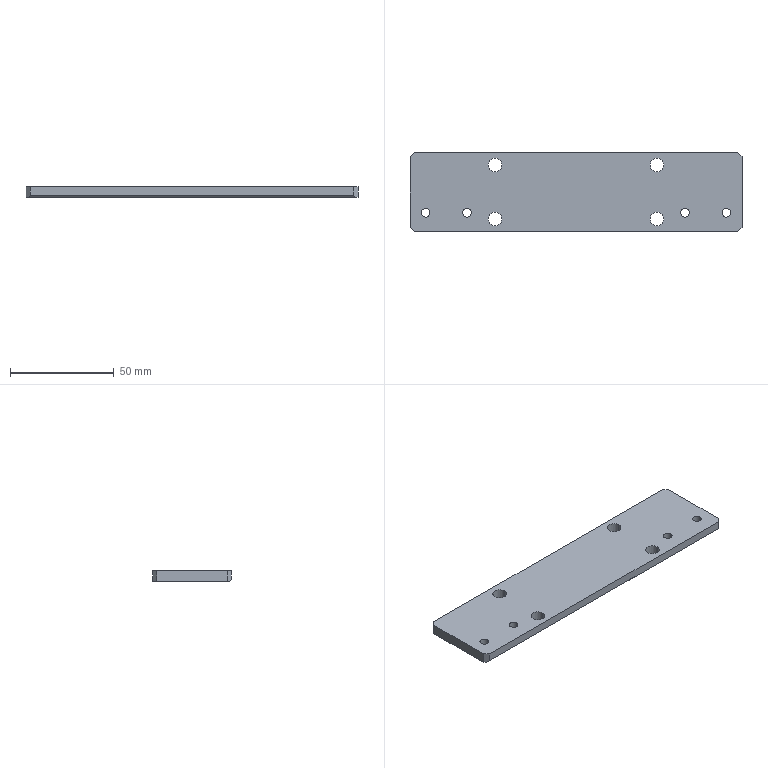Part | SolidWorks | features BaseBody 1 | 1 solid | 27 faces | box 160 x 38 x 5 mm | volume 29320 mm3 | cylinder 16 | plane 11 | commonest cylinder face diameters 4.2 x8 6.6 x8
STEP:
#1=CARTESIAN_POINT('',(35.7,-13.,5.));
#2=VERTEX_POINT('',#1);
#3=CARTESIAN_POINT('',(42.3,-13.,5.));
#4=VERTEX_POINT('',#3);
#5=CARTESIAN_POINT('',(39.,-13.,5.));
#6=DIRECTION('',(0.,0.,1.));
#7=DIRECTION('',(-1.,0.,0.));
#8=AXIS2_PLACEMENT_3D('',#5,#6,#7);
#9=CIRCLE('',#8,3.3);
#10=EDGE_CURVE('',#2,#4,#9,.T.);
#11=ORIENTED_EDGE('',*,*,#10,.T.);
#12=CARTESIAN_POINT('',(42.3,-13.,0.));
#13=VERTEX_POINT('',#12);
#14=CARTESIAN_POINT('',(42.3,-13.,0.));
#15=DIRECTION('',(0.,0.,-1.));
#16=VECTOR('',#15,1000.);
#17=LINE('',#14,#16);
#18=EDGE_CURVE('',#4,#13,#17,.T.);
#19=ORIENTED_EDGE('',*,*,#18,.T.);
#20=CARTESIAN_POINT('',(35.7,-13.,0.));
#21=VERTEX_POINT('',#20);
#22=CARTESIAN_POINT('',(39.,-13.,0.));
#23=DIRECTION('',(0.,0.,1.));
#24=DIRECTION('',(-1.,0.,0.));
#25=AXIS2_PLACEMENT_3D('',#22,#23,#24);
#26=CIRCLE('',#25,3.3);
#27=EDGE_CURVE('',#21,#13,#26,.T.);
#28=ORIENTED_EDGE('',*,*,#27,.F.);
#29=CARTESIAN_POINT('',(35.7,-13.,0.));
#30=DIRECTION('',(0.,0.,-1.));
#31=VECTOR('',#30,1000.);
#32=LINE('',#29,#31);
#33=EDGE_CURVE('',#2,#21,#32,.T.);
#34=ORIENTED_EDGE('',*,*,#33,.F.);
#35=EDGE_LOOP('',(#11,#19,#28,#34));
#36=FACE_OUTER_BOUND('',#35,.T.);
#37=CARTESIAN_POINT('',(39.,-13.,0.));
#38=DIRECTION('',(0.,0.,-1.));
#39=DIRECTION('',(-1.,0.,0.));
#40=AXIS2_PLACEMENT_3D('',#37,#38,#39);
#41=CYLINDRICAL_SURFACE('',#40,3.3);
#42=ADVANCED_FACE('',(#36),#41,.F.);
#43=CARTESIAN_POINT('',(-42.3,-13.,5.));
#44=VERTEX_POINT('',#43);
#45=CARTESIAN_POINT('',(-35.7,-13.,5.));
#46=VERTEX_POINT('',#45);
#47=CARTESIAN_POINT('',(-39.,-13.,5.));
#48=DIRECTION('',(0.,0.,1.));
#49=DIRECTION('',(-1.,0.,0.));
#50=AXIS2_PLACEMENT_3D('',#47,#48,#49);
#51=CIRCLE('',#50,3.3);
#52=EDGE_CURVE('',#44,#46,#51,.T.);
#53=ORIENTED_EDGE('',*,*,#52,.T.);
#54=CARTESIAN_POINT('',(-35.7,-13.,0.));
#55=VERTEX_POINT('',#54);
#56=CARTESIAN_POINT('',(-35.7,-13.,0.));
#57=DIRECTION('',(0.,0.,-1.));
#58=VECTOR('',#57,1000.);
#59=LINE('',#56,#58);
#60=EDGE_CURVE('',#46,#55,#59,.T.);
#61=ORIENTED_EDGE('',*,*,#60,.T.);
#62=CARTESIAN_POINT('',(-42.3,-13.,0.));
#63=VERTEX_POINT('',#62);
#64=CARTESIAN_POINT('',(-39.,-13.,0.));
#65=DIRECTION('',(0.,0.,1.));
#66=DIRECTION('',(-1.,0.,0.));
#67=AXIS2_PLACEMENT_3D('',#64,#65,#66);
#68=CIRCLE('',#67,3.3);
#69=EDGE_CURVE('',#63,#55,#68,.T.);
#70=ORIENTED_EDGE('',*,*,#69,.F.);
#71=CARTESIAN_POINT('',(-42.3,-13.,0.));
#72=DIRECTION('',(0.,0.,-1.));
#73=VECTOR('',#72,1000.);
#74=LINE('',#71,#73);
#75=EDGE_CURVE('',#44,#63,#74,.T.);
#76=ORIENTED_EDGE('',*,*,#75,.F.);
#77=EDGE_LOOP('',(#53,#61,#70,#76));
#78=FACE_OUTER_BOUND('',#77,.T.);
#79=CARTESIAN_POINT('',(-39.,-13.,0.));
#80=DIRECTION('',(0.,0.,-1.));
#81=DIRECTION('',(-1.,0.,0.));
#82=AXIS2_PLACEMENT_3D('',#79,#80,#81);
#83=CYLINDRICAL_SURFACE('',#82,3.3);
#84=ADVANCED_FACE('',(#78),#83,.F.);
#85=CARTESIAN_POINT('',(-42.3,13.,5.));
#86=VERTEX_POINT('',#85);
#87=CARTESIAN_POINT('',(-35.7,13.,5.));
#88=VERTEX_POINT('',#87);
#89=CARTESIAN_POINT('',(-39.,13.,5.));
#90=DIRECTION('',(0.,0.,1.));
#91=DIRECTION('',(-1.,0.,0.));
#92=AXIS2_PLACEMENT_3D('',#89,#90,#91);
#93=CIRCLE('',#92,3.3);
#94=EDGE_CURVE('',#86,#88,#93,.T.);
#95=ORIENTED_EDGE('',*,*,#94,.T.);
#96=CARTESIAN_POINT('',(-35.7,13.,0.));
#97=VERTEX_POINT('',#96);
#98=CARTESIAN_POINT('',(-35.7,13.,0.));
#99=DIRECTION('',(0.,0.,-1.));
#100=VECTOR('',#99,1000.);
#101=LINE('',#98,#100);
#102=EDGE_CURVE('',#88,#97,#101,.T.);
#103=ORIENTED_EDGE('',*,*,#102,.T.);
#104=CARTESIAN_POINT('',(-42.3,13.,0.));
#105=VERTEX_POINT('',#104);
#106=CARTESIAN_POINT('',(-39.,13.,0.));
#107=DIRECTION('',(0.,0.,1.));
#108=DIRECTION('',(-1.,0.,0.));
#109=AXIS2_PLACEMENT_3D('',#106,#107,#108);
#110=CIRCLE('',#109,3.3);
#111=EDGE_CURVE('',#105,#97,#110,.T.);
#112=ORIENTED_EDGE('',*,*,#111,.F.);
#113=CARTESIAN_POINT('',(-42.3,13.,0.));
#114=DIRECTION('',(0.,0.,-1.));
#115=VECTOR('',#114,1000.);
#116=LINE('',#113,#115);
#117=EDGE_CURVE('',#86,#105,#116,.T.);
#118=ORIENTED_EDGE('',*,*,#117,.F.);
#119=EDGE_LOOP('',(#95,#103,#112,#118));
#120=FACE_OUTER_BOUND('',#119,.T.);
#121=CARTESIAN_POINT('',(-39.,13.,0.));
#122=DIRECTION('',(0.,0.,-1.));
#123=DIRECTION('',(-1.,0.,0.));
#124=AXIS2_PLACEMENT_3D('',#121,#122,#123);
#125=CYLINDRICAL_SURFACE('',#124,3.3);
#126=ADVANCED_FACE('',(#120),#125,.F.);
#127=CARTESIAN_POINT('',(35.7,13.,5.));
#128=VERTEX_POINT('',#127);
#129=CARTESIAN_POINT('',(42.3,13.,5.));
#130=VERTEX_POINT('',#129);
#131=CARTESIAN_POINT('',(39.,13.,5.));
#132=DIRECTION('',(0.,0.,1.));
#133=DIRECTION('',(-1.,0.,0.));
#134=AXIS2_PLACEMENT_3D('',#131,#132,#133);
#135=CIRCLE('',#134,3.3);
#136=EDGE_CURVE('',#128,#130,#135,.T.);
#137=ORIENTED_EDGE('',*,*,#136,.T.);
#138=CARTESIAN_POINT('',(42.3,13.,0.));
#139=VERTEX_POINT('',#138);
#140=CARTESIAN_POINT('',(42.3,13.,0.));
#141=DIRECTION('',(0.,0.,-1.));
#142=VECTOR('',#141,1000.);
#143=LINE('',#140,#142);
#144=EDGE_CURVE('',#130,#139,#143,.T.);
#145=ORIENTED_EDGE('',*,*,#144,.T.);
#146=CARTESIAN_POINT('',(35.7,13.,0.));
#147=VERTEX_POINT('',#146);
#148=CARTESIAN_POINT('',(39.,13.,0.));
#149=DIRECTION('',(0.,0.,1.));
#150=DIRECTION('',(-1.,0.,0.));
#151=AXIS2_PLACEMENT_3D('',#148,#149,#150);
#152=CIRCLE('',#151,3.3);
#153=EDGE_CURVE('',#147,#139,#152,.T.);
#154=ORIENTED_EDGE('',*,*,#153,.F.);
#155=CARTESIAN_POINT('',(35.7,13.,0.));
#156=DIRECTION('',(0.,0.,-1.));
#157=VECTOR('',#156,1000.);
#158=LINE('',#155,#157);
#159=EDGE_CURVE('',#128,#147,#158,.T.);
#160=ORIENTED_EDGE('',*,*,#159,.F.);
#161=EDGE_LOOP('',(#137,#145,#154,#160));
#162=FACE_OUTER_BOUND('',#161,.T.);
#163=CARTESIAN_POINT('',(39.,13.,0.));
#164=DIRECTION('',(0.,0.,-1.));
#165=DIRECTION('',(-1.,0.,0.));
#166=AXIS2_PLACEMENT_3D('',#163,#164,#165);
#167=CYLINDRICAL_SURFACE('',#166,3.3);
#168=ADVANCED_FACE('',(#162),#167,.F.);
#169=CARTESIAN_POINT('',(-74.6,-10.,5.));
#170=VERTEX_POINT('',#169);
#171=CARTESIAN_POINT('',(-70.4,-10.,5.));
#172=VERTEX_POINT('',#171);
#173=CARTESIAN_POINT('',(-72.5,-10.,5.));
#174=DIRECTION('',(0.,0.,1.));
#175=DIRECTION('',(-1.,0.,0.));
#176=AXIS2_PLACEMENT_3D('',#173,#174,#175);
#177=CIRCLE('',#176,2.1);
#178=EDGE_CURVE('',#170,#172,#177,.T.);
#179=ORIENTED_EDGE('',*,*,#178,.T.);
#180=CARTESIAN_POINT('',(-70.4,-10.,0.));
#181=VERTEX_POINT('',#180);
#182=CARTESIAN_POINT('',(-70.4,-10.,0.));
#183=DIRECTION('',(0.,0.,-1.));
#184=VECTOR('',#183,1000.);
#185=LINE('',#182,#184);
#186=EDGE_CURVE('',#172,#181,#185,.T.);
#187=ORIENTED_EDGE('',*,*,#186,.T.);
#188=CARTESIAN_POINT('',(-74.6,-10.,0.));
#189=VERTEX_POINT('',#188);
#190=CARTESIAN_POINT('',(-72.5,-10.,0.));
#191=DIRECTION('',(0.,0.,1.));
#192=DIRECTION('',(-1.,0.,0.));
#193=AXIS2_PLACEMENT_3D('',#190,#191,#192);
#194=CIRCLE('',#193,2.1);
#195=EDGE_CURVE('',#189,#181,#194,.T.);
#196=ORIENTED_EDGE('',*,*,#195,.F.);
#197=CARTESIAN_POINT('',(-74.6,-10.,0.));
#198=DIRECTION('',(0.,0.,-1.));
#199=VECTOR('',#198,1000.);
#200=LINE('',#197,#199);
#201=EDGE_CURVE('',#170,#189,#200,.T.);
#202=ORIENTED_EDGE('',*,*,#201,.F.);
#203=EDGE_LOOP('',(#179,#187,#196,#202));
#204=FACE_OUTER_BOUND('',#203,.T.);
#205=CARTESIAN_POINT('',(-72.5,-10.,0.));
#206=DIRECTION('',(0.,0.,-1.));
#207=DIRECTION('',(-1.,0.,0.));
#208=AXIS2_PLACEMENT_3D('',#205,#206,#207);
#209=CYLINDRICAL_SURFACE('',#208,2.1);
#210=ADVANCED_FACE('',(#204),#209,.F.);
#211=CARTESIAN_POINT('',(70.4,-10.,5.));
#212=VERTEX_POINT('',#211);
#213=CARTESIAN_POINT('',(74.6,-10.,5.));
#214=VERTEX_POINT('',#213);
#215=CARTESIAN_POINT('',(72.5,-10.,5.));
#216=DIRECTION('',(0.,0.,1.));
#217=DIRECTION('',(-1.,0.,0.));
#218=AXIS2_PLACEMENT_3D('',#215,#216,#217);
#219=CIRCLE('',#218,2.1);
#220=EDGE_CURVE('',#212,#214,#219,.T.);
#221=ORIENTED_EDGE('',*,*,#220,.T.);
#222=CARTESIAN_POINT('',(74.6,-10.,0.));
#223=VERTEX_POINT('',#222);
#224=CARTESIAN_POINT('',(74.6,-10.,0.));
#225=DIRECTION('',(0.,0.,-1.));
#226=VECTOR('',#225,1000.);
#227=LINE('',#224,#226);
#228=EDGE_CURVE('',#214,#223,#227,.T.);
#229=ORIENTED_EDGE('',*,*,#228,.T.);
#230=CARTESIAN_POINT('',(70.4,-10.,0.));
#231=VERTEX_POINT('',#230);
#232=CARTESIAN_POINT('',(72.5,-10.,0.));
#233=DIRECTION('',(0.,0.,1.));
#234=DIRECTION('',(-1.,0.,0.));
#235=AXIS2_PLACEMENT_3D('',#232,#233,#234);
#236=CIRCLE('',#235,2.1);
#237=EDGE_CURVE('',#231,#223,#236,.T.);
#238=ORIENTED_EDGE('',*,*,#237,.F.);
#239=CARTESIAN_POINT('',(70.4,-10.,0.));
#240=DIRECTION('',(0.,0.,-1.));
#241=VECTOR('',#240,1000.);
#242=LINE('',#239,#241);
#243=EDGE_CURVE('',#212,#231,#242,.T.);
#244=ORIENTED_EDGE('',*,*,#243,.F.);
#245=EDGE_LOOP('',(#221,#229,#238,#244));
#246=FACE_OUTER_BOUND('',#245,.T.);
#247=CARTESIAN_POINT('',(72.5,-10.,0.));
#248=DIRECTION('',(0.,0.,-1.));
#249=DIRECTION('',(-1.,0.,0.));
#250=AXIS2_PLACEMENT_3D('',#247,#248,#249);
#251=CYLINDRICAL_SURFACE('',#250,2.1);
#252=ADVANCED_FACE('',(#246),#251,.F.);
#253=CARTESIAN_POINT('',(-54.6,-10.,5.));
#254=VERTEX_POINT('',#253);
#255=CARTESIAN_POINT('',(-50.4,-10.,5.));
#256=VERTEX_POINT('',#255);
#257=CARTESIAN_POINT('',(-52.5,-10.,5.));
#258=DIRECTION('',(0.,0.,1.));
#259=DIRECTION('',(-1.,0.,0.));
#260=AXIS2_PLACEMENT_3D('',#257,#258,#259);
#261=CIRCLE('',#260,2.1);
#262=EDGE_CURVE('',#254,#256,#261,.T.);
#263=ORIENTED_EDGE('',*,*,#262,.T.);
#264=CARTESIAN_POINT('',(-50.4,-10.,0.));
#265=VERTEX_POINT('',#264);
#266=CARTESIAN_POINT('',(-50.4,-10.,0.));
#267=DIRECTION('',(0.,0.,-1.));
#268=VECTOR('',#267,1000.);
#269=LINE('',#266,#268);
#270=EDGE_CURVE('',#256,#265,#269,.T.);
#271=ORIENTED_EDGE('',*,*,#270,.T.);
#272=CARTESIAN_POINT('',(-54.6,-10.,0.));
#273=VERTEX_POINT('',#272);
#274=CARTESIAN_POINT('',(-52.5,-10.,0.));
#275=DIRECTION('',(0.,0.,1.));
#276=DIRECTION('',(-1.,0.,0.));
#277=AXIS2_PLACEMENT_3D('',#274,#275,#276);
#278=CIRCLE('',#277,2.1);
#279=EDGE_CURVE('',#273,#265,#278,.T.);
#280=ORIENTED_EDGE('',*,*,#279,.F.);
#281=CARTESIAN_POINT('',(-54.6,-10.,0.));
#282=DIRECTION('',(0.,0.,-1.));
#283=VECTOR('',#282,1000.);
#284=LINE('',#281,#283);
#285=EDGE_CURVE('',#254,#273,#284,.T.);
#286=ORIENTED_EDGE('',*,*,#285,.F.);
#287=EDGE_LOOP('',(#263,#271,#280,#286));
#288=FACE_OUTER_BOUND('',#287,.T.);
#289=CARTESIAN_POINT('',(-52.5,-10.,0.));
#290=DIRECTION('',(0.,0.,-1.));
#291=DIRECTION('',(-1.,0.,0.));
#292=AXIS2_PLACEMENT_3D('',#289,#290,#291);
#293=CYLINDRICAL_SURFACE('',#292,2.1);
#294=ADVANCED_FACE('',(#288),#293,.F.);
#295=CARTESIAN_POINT('',(50.4,-10.,5.));
#296=VERTEX_POINT('',#295);
#297=CARTESIAN_POINT('',(54.6,-10.,5.));
#298=VERTEX_POINT('',#297);
#299=CARTESIAN_POINT('',(52.5,-10.,5.));
#300=DIRECTION('',(0.,0.,1.));
#301=DIRECTION('',(-1.,0.,0.));
#302=AXIS2_PLACEMENT_3D('',#299,#300,#301);
#303=CIRCLE('',#302,2.1);
#304=EDGE_CURVE('',#296,#298,#303,.T.);
#305=ORIENTED_EDGE('',*,*,#304,.T.);
#306=CARTESIAN_POINT('',(54.6,-10.,0.));
#307=VERTEX_POINT('',#306);
#308=CARTESIAN_POINT('',(54.6,-10.,0.));
#309=DIRECTION('',(0.,0.,-1.));
#310=VECTOR('',#309,1000.);
#311=LINE('',#308,#310);
#312=EDGE_CURVE('',#298,#307,#311,.T.);
#313=ORIENTED_EDGE('',*,*,#312,.T.);
#314=CARTESIAN_POINT('',(50.4,-10.,0.));
#315=VERTEX_POINT('',#314);
#316=CARTESIAN_POINT('',(52.5,-10.,0.));
#317=DIRECTION('',(0.,0.,1.));
#318=DIRECTION('',(-1.,0.,0.));
#319=AXIS2_PLACEMENT_3D('',#316,#317,#318);
#320=CIRCLE('',#319,2.1);
#321=EDGE_CURVE('',#315,#307,#320,.T.);
#322=ORIENTED_EDGE('',*,*,#321,.F.);
#323=CARTESIAN_POINT('',(50.4,-10.,0.));
#324=DIRECTION('',(0.,0.,-1.));
#325=VECTOR('',#324,1000.);
#326=LINE('',#323,#325);
#327=EDGE_CURVE('',#296,#315,#326,.T.);
#328=ORIENTED_EDGE('',*,*,#327,.F.);
#329=EDGE_LOOP('',(#305,#313,#322,#328));
#330=FACE_OUTER_BOUND('',#329,.T.);
#331=CARTESIAN_POINT('',(52.5,-10.,0.));
#332=DIRECTION('',(0.,0.,-1.));
#333=DIRECTION('',(-1.,0.,0.));
#334=AXIS2_PLACEMENT_3D('',#331,#332,#333);
#335=CYLINDRICAL_SURFACE('',#334,2.1);
#336=ADVANCED_FACE('',(#330),#335,.F.);
#337=CARTESIAN_POINT('',(80.,-17.,5.));
#338=VERTEX_POINT('',#337);
#339=CARTESIAN_POINT('',(78.,-19.,5.));
#340=VERTEX_POINT('',#339);
#341=CARTESIAN_POINT('',(80.,-17.,5.));
#342=DIRECTION('',(-0.7071,-0.7071,0.));
#343=VECTOR('',#342,1000.);
#344=LINE('',#341,#343);
#345=EDGE_CURVE('',#338,#340,#344,.T.);
#346=ORIENTED_EDGE('',*,*,#345,.F.);
#347=CARTESIAN_POINT('',(80.,17.,5.));
#348=VERTEX_POINT('',#347);
#349=CARTESIAN_POINT('',(80.,0.,5.));
#350=DIRECTION('',(0.,-1.,0.));
#351=VECTOR('',#350,1000.);
#352=LINE('',#349,#351);
#353=EDGE_CURVE('',#348,#338,#352,.T.);
#354=ORIENTED_EDGE('',*,*,#353,.F.);
#355=CARTESIAN_POINT('',(78.,19.,5.));
#356=VERTEX_POINT('',#355);
#357=CARTESIAN_POINT('',(78.,19.,5.));
#358=DIRECTION('',(0.7071,-0.7071,0.));
#359=VECTOR('',#358,1000.);
#360=LINE('',#357,#359);
#361=EDGE_CURVE('',#356,#348,#360,.T.);
#362=ORIENTED_EDGE('',*,*,#361,.F.);
#363=CARTESIAN_POINT('',(-78.,19.,5.));
#364=VERTEX_POINT('',#363);
#365=CARTESIAN_POINT('',(0.,19.,5.));
#366=DIRECTION('',(1.,0.,0.));
#367=VECTOR('',#366,1000.);
#368=LINE('',#365,#367);
#369=EDGE_CURVE('',#364,#356,#368,.T.);
#370=ORIENTED_EDGE('',*,*,#369,.F.);
#371=CARTESIAN_POINT('',(-80.,17.,5.));
#372=VERTEX_POINT('',#371);
#373=CARTESIAN_POINT('',(-80.,17.,5.));
#374=DIRECTION('',(0.7071,0.7071,0.));
#375=VECTOR('',#374,1000.);
#376=LINE('',#373,#375);
#377=EDGE_CURVE('',#372,#364,#376,.T.);
#378=ORIENTED_EDGE('',*,*,#377,.F.);
#379=CARTESIAN_POINT('',(-80.,-17.,5.));
#380=VERTEX_POINT('',#379);
#381=CARTESIAN_POINT('',(-80.,0.,5.));
#382=DIRECTION('',(0.,1.,0.));
#383=VECTOR('',#382,1000.);
#384=LINE('',#381,#383);
#385=EDGE_CURVE('',#380,#372,#384,.T.);
#386=ORIENTED_EDGE('',*,*,#385,.F.);
#387=CARTESIAN_POINT('',(-78.,-19.,5.));
#388=VERTEX_POINT('',#387);
#389=CARTESIAN_POINT('',(-78.,-19.,5.));
#390=DIRECTION('',(-0.7071,0.7071,0.));
#391=VECTOR('',#390,1000.);
#392=LINE('',#389,#391);
#393=EDGE_CURVE('',#388,#380,#392,.T.);
#394=ORIENTED_EDGE('',*,*,#393,.F.);
#395=CARTESIAN_POINT('',(0.,-19.,5.));
#396=DIRECTION('',(-1.,0.,0.));
#397=VECTOR('',#396,1000.);
#398=LINE('',#395,#397);
#399=EDGE_CURVE('',#340,#388,#398,.T.);
#400=ORIENTED_EDGE('',*,*,#399,.F.);
#401=EDGE_LOOP('',(#346,#354,#362,#370,#378,#386,#394,#400));
#402=FACE_OUTER_BOUND('',#401,.T.);
#403=ORIENTED_EDGE('',*,*,#10,.F.);
#404=CARTESIAN_POINT('',(39.,-13.,5.));
#405=DIRECTION('',(0.,0.,1.));
#406=DIRECTION('',(-1.,0.,0.));
#407=AXIS2_PLACEMENT_3D('',#404,#405,#406);
#408=CIRCLE('',#407,3.3);
#409=EDGE_CURVE('',#4,#2,#408,.T.);
#410=ORIENTED_EDGE('',*,*,#409,.F.);
#411=EDGE_LOOP('',(#403,#410));
#412=FACE_BOUND('',#411,.T.);
#413=ORIENTED_EDGE('',*,*,#52,.F.);
#414=CARTESIAN_POINT('',(-39.,-13.,5.));
#415=DIRECTION('',(0.,0.,1.));
#416=DIRECTION('',(-1.,0.,0.));
#417=AXIS2_PLACEMENT_3D('',#414,#415,#416);
#418=CIRCLE('',#417,3.3);
#419=EDGE_CURVE('',#46,#44,#418,.T.);
#420=ORIENTED_EDGE('',*,*,#419,.F.);
#421=EDGE_LOOP('',(#413,#420));
#422=FACE_BOUND('',#421,.T.);
#423=ORIENTED_EDGE('',*,*,#94,.F.);
#424=CARTESIAN_POINT('',(-39.,13.,5.));
#425=DIRECTION('',(0.,0.,1.));
#426=DIRECTION('',(-1.,0.,0.));
#427=AXIS2_PLACEMENT_3D('',#424,#425,#426);
#428=CIRCLE('',#427,3.3);
#429=EDGE_CURVE('',#88,#86,#428,.T.);
#430=ORIENTED_EDGE('',*,*,#429,.F.);
#431=EDGE_LOOP('',(#423,#430));
#432=FACE_BOUND('',#431,.T.);
#433=ORIENTED_EDGE('',*,*,#136,.F.);
#434=CARTESIAN_POINT('',(39.,13.,5.));
#435=DIRECTION('',(0.,0.,1.));
#436=DIRECTION('',(-1.,0.,0.));
#437=AXIS2_PLACEMENT_3D('',#434,#435,#436);
#438=CIRCLE('',#437,3.3);
#439=EDGE_CURVE('',#130,#128,#438,.T.);
#440=ORIENTED_EDGE('',*,*,#439,.F.);
#441=EDGE_LOOP('',(#433,#440));
#442=FACE_BOUND('',#441,.T.);
#443=ORIENTED_EDGE('',*,*,#178,.F.);
#444=CARTESIAN_POINT('',(-72.5,-10.,5.));
#445=DIRECTION('',(0.,0.,1.));
#446=DIRECTION('',(-1.,0.,0.));
#447=AXIS2_PLACEMENT_3D('',#444,#445,#446);
#448=CIRCLE('',#447,2.1);
#449=EDGE_CURVE('',#172,#170,#448,.T.);
#450=ORIENTED_EDGE('',*,*,#449,.F.);
#451=EDGE_LOOP('',(#443,#450));
#452=FACE_BOUND('',#451,.T.);
#453=ORIENTED_EDGE('',*,*,#220,.F.);
#454=CARTESIAN_POINT('',(72.5,-10.,5.));
#455=DIRECTION('',(0.,0.,1.));
#456=DIRECTION('',(-1.,0.,0.));
#457=AXIS2_PLACEMENT_3D('',#454,#455,#456);
#458=CIRCLE('',#457,2.1);
#459=EDGE_CURVE('',#214,#212,#458,.T.);
#460=ORIENTED_EDGE('',*,*,#459,.F.);
#461=EDGE_LOOP('',(#453,#460));
#462=FACE_BOUND('',#461,.T.);
#463=ORIENTED_EDGE('',*,*,#262,.F.);
#464=CARTESIAN_POINT('',(-52.5,-10.,5.));
#465=DIRECTION('',(0.,0.,1.));
#466=DIRECTION('',(-1.,0.,0.));
#467=AXIS2_PLACEMENT_3D('',#464,#465,#466);
#468=CIRCLE('',#467,2.1);
#469=EDGE_CURVE('',#256,#254,#468,.T.);
#470=ORIENTED_EDGE('',*,*,#469,.F.);
#471=EDGE_LOOP('',(#463,#470));
#472=FACE_BOUND('',#471,.T.);
#473=ORIENTED_EDGE('',*,*,#304,.F.);
#474=CARTESIAN_POINT('',(52.5,-10.,5.));
#475=DIRECTION('',(0.,0.,1.));
#476=DIRECTION('',(-1.,0.,0.));
#477=AXIS2_PLACEMENT_3D('',#474,#475,#476);
#478=CIRCLE('',#477,2.1);
#479=EDGE_CURVE('',#298,#296,#478,.T.);
#480=ORIENTED_EDGE('',*,*,#479,.F.);
#481=EDGE_LOOP('',(#473,#480));
#482=FACE_BOUND('',#481,.T.);
#483=CARTESIAN_POINT('',(0.,0.,5.));
#484=DIRECTION('',(0.,0.,-1.));
#485=DIRECTION('',(-1.,0.,0.));
#486=AXIS2_PLACEMENT_3D('',#483,#484,#485);
#487=PLANE('',#486);
#488=ADVANCED_FACE('',(#402,#412,#422,#432,#442,#452,#462,#472,#482),#487,.F.);
#489=CARTESIAN_POINT('',(78.,-19.,1.));
#490=VERTEX_POINT('',#489);
#491=CARTESIAN_POINT('',(78.,-19.,5.));
#492=DIRECTION('',(0.,0.,-1.));
#493=VECTOR('',#492,1000.);
#494=LINE('',#491,#493);
#495=EDGE_CURVE('',#340,#490,#494,.T.);
#496=ORIENTED_EDGE('',*,*,#495,.F.);
#497=ORIENTED_EDGE('',*,*,#399,.T.);
#498=CARTESIAN_POINT('',(-78.,-19.,1.));
#499=VERTEX_POINT('',#498);
#500=CARTESIAN_POINT('',(-78.,-19.,5.));
#501=DIRECTION('',(0.,0.,1.));
#502=VECTOR('',#501,1000.);
#503=LINE('',#500,#502);
#504=EDGE_CURVE('',#499,#388,#503,.T.);
#505=ORIENTED_EDGE('',*,*,#504,.F.);
#506=CARTESIAN_POINT('',(-80.,-19.,1.));
#507=DIRECTION('',(-1.,0.,0.));
#508=VECTOR('',#507,1000.);
#509=LINE('',#506,#508);
#510=EDGE_CURVE('',#490,#499,#509,.T.);
#511=ORIENTED_EDGE('',*,*,#510,.F.);
#512=EDGE_LOOP('',(#496,#497,#505,#511));
#513=FACE_OUTER_BOUND('',#512,.T.);
#514=CARTESIAN_POINT('',(-80.,-19.,5.));
#515=DIRECTION('',(0.,1.,0.));
#516=DIRECTION('',(0.,0.,1.));
#517=AXIS2_PLACEMENT_3D('',#514,#515,#516);
#518=PLANE('',#517);
#519=ADVANCED_FACE('',(#513),#518,.F.);
#520=ORIENTED_EDGE('',*,*,#495,.T.);
#521=CARTESIAN_POINT('',(79.,-18.,0.));
#522=VERTEX_POINT('',#521);
#523=CARTESIAN_POINT('',(79.,-18.,0.));
#524=DIRECTION('',(-0.5774,-0.5774,0.5774));
#525=VECTOR('',#524,1000.);
#526=LINE('',#523,#525);
#527=EDGE_CURVE('',#522,#490,#526,.T.);
#528=ORIENTED_EDGE('',*,*,#527,.F.);
#529=CARTESIAN_POINT('',(80.,-17.,0.));
#530=VERTEX_POINT('',#529);
#531=CARTESIAN_POINT('',(80.,-17.,0.));
#532=DIRECTION('',(-0.7071,-0.7071,0.));
#533=VECTOR('',#532,1000.);
#534=LINE('',#531,#533);
#535=EDGE_CURVE('',#530,#522,#534,.T.);
#536=ORIENTED_EDGE('',*,*,#535,.F.);
#537=CARTESIAN_POINT('',(80.,-17.,5.));
#538=DIRECTION('',(0.,0.,-1.));
#539=VECTOR('',#538,1000.);
#540=LINE('',#537,#539);
#541=EDGE_CURVE('',#338,#530,#540,.T.);
#542=ORIENTED_EDGE('',*,*,#541,.F.);
#543=ORIENTED_EDGE('',*,*,#345,.T.);
#544=EDGE_LOOP('',(#520,#528,#536,#542,#543));
#545=FACE_OUTER_BOUND('',#544,.T.);
#546=CARTESIAN_POINT('',(80.,-17.,5.));
#547=DIRECTION('',(-0.7071,0.7071,0.));
#548=DIRECTION('',(-0.7071,-0.7071,0.));
#549=AXIS2_PLACEMENT_3D('',#546,#547,#548);
#550=PLANE('',#549);
#551=ADVANCED_FACE('',(#545),#550,.F.);
#552=ORIENTED_EDGE('',*,*,#541,.T.);
#553=CARTESIAN_POINT('',(80.,17.,0.));
#554=VERTEX_POINT('',#553);
#555=CARTESIAN_POINT('',(80.,-19.,0.));
#556=DIRECTION('',(0.,-1.,0.));
#557=VECTOR('',#556,1000.);
#558=LINE('',#555,#557);
#559=EDGE_CURVE('',#554,#530,#558,.T.);
#560=ORIENTED_EDGE('',*,*,#559,.F.);
#561=CARTESIAN_POINT('',(80.,17.,5.));
#562=DIRECTION('',(0.,0.,-1.));
#563=VECTOR('',#562,1000.);
#564=LINE('',#561,#563);
#565=EDGE_CURVE('',#348,#554,#564,.T.);
#566=ORIENTED_EDGE('',*,*,#565,.F.);
#567=ORIENTED_EDGE('',*,*,#353,.T.);
#568=EDGE_LOOP('',(#552,#560,#566,#567));
#569=FACE_OUTER_BOUND('',#568,.T.);
#570=CARTESIAN_POINT('',(80.,-19.,5.));
#571=DIRECTION('',(-1.,0.,0.));
#572=DIRECTION('',(0.,0.,1.));
#573=AXIS2_PLACEMENT_3D('',#570,#571,#572);
#574=PLANE('',#573);
#575=ADVANCED_FACE('',(#569),#574,.F.);
#576=ORIENTED_EDGE('',*,*,#565,.T.);
#577=CARTESIAN_POINT('',(78.,19.,0.));
#578=VERTEX_POINT('',#577);
#579=CARTESIAN_POINT('',(78.,19.,0.));
#580=DIRECTION('',(0.7071,-0.7071,0.));
#581=VECTOR('',#580,1000.);
#582=LINE('',#579,#581);
#583=EDGE_CURVE('',#578,#554,#582,.T.);
#584=ORIENTED_EDGE('',*,*,#583,.F.);
#585=CARTESIAN_POINT('',(78.,19.,5.));
#586=DIRECTION('',(0.,0.,-1.));
#587=VECTOR('',#586,1000.);
#588=LINE('',#585,#587);
#589=EDGE_CURVE('',#356,#578,#588,.T.);
#590=ORIENTED_EDGE('',*,*,#589,.F.);
#591=ORIENTED_EDGE('',*,*,#361,.T.);
#592=EDGE_LOOP('',(#576,#584,#590,#591));
#593=FACE_OUTER_BOUND('',#592,.T.);
#594=CARTESIAN_POINT('',(78.,19.,5.));
#595=DIRECTION('',(-0.7071,-0.7071,0.));
#596=DIRECTION('',(0.7071,-0.7071,0.));
#597=AXIS2_PLACEMENT_3D('',#594,#595,#596);
#598=PLANE('',#597);
#599=ADVANCED_FACE('',(#593),#598,.F.);
#600=ORIENTED_EDGE('',*,*,#589,.T.);
#601=CARTESIAN_POINT('',(-78.,19.,0.));
#602=VERTEX_POINT('',#601);
#603=CARTESIAN_POINT('',(-80.,19.,0.));
#604=DIRECTION('',(1.,0.,0.));
#605=VECTOR('',#604,1000.);
#606=LINE('',#603,#605);
#607=EDGE_CURVE('',#602,#578,#606,.T.);
#608=ORIENTED_EDGE('',*,*,#607,.F.);
#609=CARTESIAN_POINT('',(-78.,19.,5.));
#610=DIRECTION('',(0.,0.,-1.));
#611=VECTOR('',#610,1000.);
#612=LINE('',#609,#611);
#613=EDGE_CURVE('',#364,#602,#612,.T.);
#614=ORIENTED_EDGE('',*,*,#613,.F.);
#615=ORIENTED_EDGE('',*,*,#369,.T.);
#616=EDGE_LOOP('',(#600,#608,#614,#615));
#617=FACE_OUTER_BOUND('',#616,.T.);
#618=CARTESIAN_POINT('',(-80.,19.,5.));
#619=DIRECTION('',(0.,-1.,0.));
#620=DIRECTION('',(0.,0.,-1.));
#621=AXIS2_PLACEMENT_3D('',#618,#619,#620);
#622=PLANE('',#621);
#623=ADVANCED_FACE('',(#617),#622,.F.);
#624=ORIENTED_EDGE('',*,*,#613,.T.);
#625=CARTESIAN_POINT('',(-80.,17.,0.));
#626=VERTEX_POINT('',#625);
#627=CARTESIAN_POINT('',(-80.,17.,0.));
#628=DIRECTION('',(0.7071,0.7071,0.));
#629=VECTOR('',#628,1000.);
#630=LINE('',#627,#629);
#631=EDGE_CURVE('',#626,#602,#630,.T.);
#632=ORIENTED_EDGE('',*,*,#631,.F.);
#633=CARTESIAN_POINT('',(-80.,17.,5.));
#634=DIRECTION('',(0.,0.,-1.));
#635=VECTOR('',#634,1000.);
#636=LINE('',#633,#635);
#637=EDGE_CURVE('',#372,#626,#636,.T.);
#638=ORIENTED_EDGE('',*,*,#637,.F.);
#639=ORIENTED_EDGE('',*,*,#377,.T.);
#640=EDGE_LOOP('',(#624,#632,#638,#639));
#641=FACE_OUTER_BOUND('',#640,.T.);
#642=CARTESIAN_POINT('',(-80.,17.,5.));
#643=DIRECTION('',(0.7071,-0.7071,0.));
#644=DIRECTION('',(0.7071,0.7071,0.));
#645=AXIS2_PLACEMENT_3D('',#642,#643,#644);
#646=PLANE('',#645);
#647=ADVANCED_FACE('',(#641),#646,.F.);
#648=ORIENTED_EDGE('',*,*,#637,.T.);
#649=CARTESIAN_POINT('',(-80.,-17.,0.));
#650=VERTEX_POINT('',#649);
#651=CARTESIAN_POINT('',(-80.,-19.,0.));
#652=DIRECTION('',(0.,1.,0.));
#653=VECTOR('',#652,1000.);
#654=LINE('',#651,#653);
#655=EDGE_CURVE('',#650,#626,#654,.T.);
#656=ORIENTED_EDGE('',*,*,#655,.F.);
#657=CARTESIAN_POINT('',(-80.,-17.,5.));
#658=DIRECTION('',(0.,0.,-1.));
#659=VECTOR('',#658,1000.);
#660=LINE('',#657,#659);
#661=EDGE_CURVE('',#380,#650,#660,.T.);
#662=ORIENTED_EDGE('',*,*,#661,.F.);
#663=ORIENTED_EDGE('',*,*,#385,.T.);
#664=EDGE_LOOP('',(#648,#656,#662,#663));
#665=FACE_OUTER_BOUND('',#664,.T.);
#666=CARTESIAN_POINT('',(-80.,-19.,5.));
#667=DIRECTION('',(1.,0.,0.));
#668=DIRECTION('',(0.,0.,-1.));
#669=AXIS2_PLACEMENT_3D('',#666,#667,#668);
#670=PLANE('',#669);
#671=ADVANCED_FACE('',(#665),#670,.F.);
#672=ORIENTED_EDGE('',*,*,#661,.T.);
#673=CARTESIAN_POINT('',(-79.,-18.,0.));
#674=VERTEX_POINT('',#673);
#675=CARTESIAN_POINT('',(-78.,-19.,0.));
#676=DIRECTION('',(-0.7071,0.7071,0.));
#677=VECTOR('',#676,1000.);
#678=LINE('',#675,#677);
#679=EDGE_CURVE('',#674,#650,#678,.T.);
#680=ORIENTED_EDGE('',*,*,#679,.F.);
#681=CARTESIAN_POINT('',(-78.,-19.,1.));
#682=DIRECTION('',(-0.5774,0.5774,-0.5774));
#683=VECTOR('',#682,1000.);
#684=LINE('',#681,#683);
#685=EDGE_CURVE('',#499,#674,#684,.T.);
#686=ORIENTED_EDGE('',*,*,#685,.F.);
#687=ORIENTED_EDGE('',*,*,#504,.T.);
#688=ORIENTED_EDGE('',*,*,#393,.T.);
#689=EDGE_LOOP('',(#672,#680,#686,#687,#688));
#690=FACE_OUTER_BOUND('',#689,.T.);
#691=CARTESIAN_POINT('',(-78.,-19.,5.));
#692=DIRECTION('',(0.7071,0.7071,0.));
#693=DIRECTION('',(-0.7071,0.7071,0.));
#694=AXIS2_PLACEMENT_3D('',#691,#692,#693);
#695=PLANE('',#694);
#696=ADVANCED_FACE('',(#690),#695,.F.);
#697=ORIENTED_EDGE('',*,*,#18,.F.);
#698=ORIENTED_EDGE('',*,*,#409,.T.);
#699=ORIENTED_EDGE('',*,*,#33,.T.);
#700=CARTESIAN_POINT('',(39.,-13.,0.));
#701=DIRECTION('',(0.,0.,1.));
#702=DIRECTION('',(-1.,0.,0.));
#703=AXIS2_PLACEMENT_3D('',#700,#701,#702);
#704=CIRCLE('',#703,3.3);
#705=EDGE_CURVE('',#13,#21,#704,.T.);
#706=ORIENTED_EDGE('',*,*,#705,.F.);
#707=EDGE_LOOP('',(#697,#698,#699,#706));
#708=FACE_OUTER_BOUND('',#707,.T.);
#709=CARTESIAN_POINT('',(39.,-13.,0.));
#710=DIRECTION('',(0.,0.,-1.));
#711=DIRECTION('',(-1.,0.,0.));
#712=AXIS2_PLACEMENT_3D('',#709,#710,#711);
#713=CYLINDRICAL_SURFACE('',#712,3.3);
#714=ADVANCED_FACE('',(#708),#713,.F.);
#715=ORIENTED_EDGE('',*,*,#60,.F.);
#716=ORIENTED_EDGE('',*,*,#419,.T.);
#717=ORIENTED_EDGE('',*,*,#75,.T.);
#718=CARTESIAN_POINT('',(-39.,-13.,0.));
#719=DIRECTION('',(0.,0.,1.));
#720=DIRECTION('',(-1.,0.,0.));
#721=AXIS2_PLACEMENT_3D('',#718,#719,#720);
#722=CIRCLE('',#721,3.3);
#723=EDGE_CURVE('',#55,#63,#722,.T.);
#724=ORIENTED_EDGE('',*,*,#723,.F.);
#725=EDGE_LOOP('',(#715,#716,#717,#724));
#726=FACE_OUTER_BOUND('',#725,.T.);
#727=CARTESIAN_POINT('',(-39.,-13.,0.));
#728=DIRECTION('',(0.,0.,-1.));
#729=DIRECTION('',(-1.,0.,0.));
#730=AXIS2_PLACEMENT_3D('',#727,#728,#729);
#731=CYLINDRICAL_SURFACE('',#730,3.3);
#732=ADVANCED_FACE('',(#726),#731,.F.);
#733=ORIENTED_EDGE('',*,*,#102,.F.);
#734=ORIENTED_EDGE('',*,*,#429,.T.);
#735=ORIENTED_EDGE('',*,*,#117,.T.);
#736=CARTESIAN_POINT('',(-39.,13.,0.));
#737=DIRECTION('',(0.,0.,1.));
#738=DIRECTION('',(-1.,0.,0.));
#739=AXIS2_PLACEMENT_3D('',#736,#737,#738);
#740=CIRCLE('',#739,3.3);
#741=EDGE_CURVE('',#97,#105,#740,.T.);
#742=ORIENTED_EDGE('',*,*,#741,.F.);
#743=EDGE_LOOP('',(#733,#734,#735,#742));
#744=FACE_OUTER_BOUND('',#743,.T.);
#745=CARTESIAN_POINT('',(-39.,13.,0.));
#746=DIRECTION('',(0.,0.,-1.));
#747=DIRECTION('',(-1.,0.,0.));
#748=AXIS2_PLACEMENT_3D('',#745,#746,#747);
#749=CYLINDRICAL_SURFACE('',#748,3.3);
#750=ADVANCED_FACE('',(#744),#749,.F.);
#751=ORIENTED_EDGE('',*,*,#144,.F.);
#752=ORIENTED_EDGE('',*,*,#439,.T.);
#753=ORIENTED_EDGE('',*,*,#159,.T.);
#754=CARTESIAN_POINT('',(39.,13.,0.));
#755=DIRECTION('',(0.,0.,1.));
#756=DIRECTION('',(-1.,0.,0.));
#757=AXIS2_PLACEMENT_3D('',#754,#755,#756);
#758=CIRCLE('',#757,3.3);
#759=EDGE_CURVE('',#139,#147,#758,.T.);
#760=ORIENTED_EDGE('',*,*,#759,.F.);
#761=EDGE_LOOP('',(#751,#752,#753,#760));
#762=FACE_OUTER_BOUND('',#761,.T.);
#763=CARTESIAN_POINT('',(39.,13.,0.));
#764=DIRECTION('',(0.,0.,-1.));
#765=DIRECTION('',(-1.,0.,0.));
#766=AXIS2_PLACEMENT_3D('',#763,#764,#765);
#767=CYLINDRICAL_SURFACE('',#766,3.3);
#768=ADVANCED_FACE('',(#762),#767,.F.);
#769=ORIENTED_EDGE('',*,*,#186,.F.);
#770=ORIENTED_EDGE('',*,*,#449,.T.);
#771=ORIENTED_EDGE('',*,*,#201,.T.);
#772=CARTESIAN_POINT('',(-72.5,-10.,0.));
#773=DIRECTION('',(0.,0.,1.));
#774=DIRECTION('',(-1.,0.,0.));
#775=AXIS2_PLACEMENT_3D('',#772,#773,#774);
#776=CIRCLE('',#775,2.1);
#777=EDGE_CURVE('',#181,#189,#776,.T.);
#778=ORIENTED_EDGE('',*,*,#777,.F.);
#779=EDGE_LOOP('',(#769,#770,#771,#778));
#780=FACE_OUTER_BOUND('',#779,.T.);
#781=CARTESIAN_POINT('',(-72.5,-10.,0.));
#782=DIRECTION('',(0.,0.,-1.));
#783=DIRECTION('',(-1.,0.,0.));
#784=AXIS2_PLACEMENT_3D('',#781,#782,#783);
#785=CYLINDRICAL_SURFACE('',#784,2.1);
#786=ADVANCED_FACE('',(#780),#785,.F.);
#787=ORIENTED_EDGE('',*,*,#228,.F.);
#788=ORIENTED_EDGE('',*,*,#459,.T.);
#789=ORIENTED_EDGE('',*,*,#243,.T.);
#790=CARTESIAN_POINT('',(72.5,-10.,0.));
#791=DIRECTION('',(0.,0.,1.));
#792=DIRECTION('',(-1.,0.,0.));
#793=AXIS2_PLACEMENT_3D('',#790,#791,#792);
#794=CIRCLE('',#793,2.1);
#795=EDGE_CURVE('',#223,#231,#794,.T.);
#796=ORIENTED_EDGE('',*,*,#795,.F.);
#797=EDGE_LOOP('',(#787,#788,#789,#796));
#798=FACE_OUTER_BOUND('',#797,.T.);
#799=CARTESIAN_POINT('',(72.5,-10.,0.));
#800=DIRECTION('',(0.,0.,-1.));
#801=DIRECTION('',(-1.,0.,0.));
#802=AXIS2_PLACEMENT_3D('',#799,#800,#801);
#803=CYLINDRICAL_SURFACE('',#802,2.1);
#804=ADVANCED_FACE('',(#798),#803,.F.);
#805=ORIENTED_EDGE('',*,*,#270,.F.);
#806=ORIENTED_EDGE('',*,*,#469,.T.);
#807=ORIENTED_EDGE('',*,*,#285,.T.);
#808=CARTESIAN_POINT('',(-52.5,-10.,0.));
#809=DIRECTION('',(0.,0.,1.));
#810=DIRECTION('',(-1.,0.,0.));
#811=AXIS2_PLACEMENT_3D('',#808,#809,#810);
#812=CIRCLE('',#811,2.1);
#813=EDGE_CURVE('',#265,#273,#812,.T.);
#814=ORIENTED_EDGE('',*,*,#813,.F.);
#815=EDGE_LOOP('',(#805,#806,#807,#814));
#816=FACE_OUTER_BOUND('',#815,.T.);
#817=CARTESIAN_POINT('',(-52.5,-10.,0.));
#818=DIRECTION('',(0.,0.,-1.));
#819=DIRECTION('',(-1.,0.,0.));
#820=AXIS2_PLACEMENT_3D('',#817,#818,#819);
#821=CYLINDRICAL_SURFACE('',#820,2.1);
#822=ADVANCED_FACE('',(#816),#821,.F.);
#823=ORIENTED_EDGE('',*,*,#312,.F.);
#824=ORIENTED_EDGE('',*,*,#479,.T.);
#825=ORIENTED_EDGE('',*,*,#327,.T.);
#826=CARTESIAN_POINT('',(52.5,-10.,0.));
#827=DIRECTION('',(0.,0.,1.));
#828=DIRECTION('',(-1.,0.,0.));
#829=AXIS2_PLACEMENT_3D('',#826,#827,#828);
#830=CIRCLE('',#829,2.1);
#831=EDGE_CURVE('',#307,#315,#830,.T.);
#832=ORIENTED_EDGE('',*,*,#831,.F.);
#833=EDGE_LOOP('',(#823,#824,#825,#832));
#834=FACE_OUTER_BOUND('',#833,.T.);
#835=CARTESIAN_POINT('',(52.5,-10.,0.));
#836=DIRECTION('',(0.,0.,-1.));
#837=DIRECTION('',(-1.,0.,0.));
#838=AXIS2_PLACEMENT_3D('',#835,#836,#837);
#839=CYLINDRICAL_SURFACE('',#838,2.1);
#840=ADVANCED_FACE('',(#834),#839,.F.);
#841=ORIENTED_EDGE('',*,*,#510,.T.);
#842=ORIENTED_EDGE('',*,*,#685,.T.);
#843=CARTESIAN_POINT('',(-80.,-18.,0.));
#844=DIRECTION('',(1.,0.,0.));
#845=VECTOR('',#844,1000.);
#846=LINE('',#843,#845);
#847=EDGE_CURVE('',#674,#522,#846,.T.);
#848=ORIENTED_EDGE('',*,*,#847,.T.);
#849=ORIENTED_EDGE('',*,*,#527,.T.);
#850=EDGE_LOOP('',(#841,#842,#848,#849));
#851=FACE_OUTER_BOUND('',#850,.T.);
#852=CARTESIAN_POINT('',(-80.,-19.,1.));
#853=DIRECTION('',(0.,-0.7071,-0.7071));
#854=DIRECTION('',(0.,0.7071,-0.7071));
#855=AXIS2_PLACEMENT_3D('',#852,#853,#854);
#856=PLANE('',#855);
#857=ADVANCED_FACE('',(#851),#856,.T.);
#858=ORIENTED_EDGE('',*,*,#607,.T.);
#859=ORIENTED_EDGE('',*,*,#583,.T.);
#860=ORIENTED_EDGE('',*,*,#559,.T.);
#861=ORIENTED_EDGE('',*,*,#535,.T.);
#862=ORIENTED_EDGE('',*,*,#847,.F.);
#863=ORIENTED_EDGE('',*,*,#679,.T.);
#864=ORIENTED_EDGE('',*,*,#655,.T.);
#865=ORIENTED_EDGE('',*,*,#631,.T.);
#866=EDGE_LOOP('',(#858,#859,#860,#861,#862,#863,#864,#865));
#867=FACE_OUTER_BOUND('',#866,.T.);
#868=ORIENTED_EDGE('',*,*,#27,.T.);
#869=ORIENTED_EDGE('',*,*,#705,.T.);
#870=EDGE_LOOP('',(#868,#869));
#871=FACE_BOUND('',#870,.T.);
#872=ORIENTED_EDGE('',*,*,#69,.T.);
#873=ORIENTED_EDGE('',*,*,#723,.T.);
#874=EDGE_LOOP('',(#872,#873));
#875=FACE_BOUND('',#874,.T.);
#876=ORIENTED_EDGE('',*,*,#111,.T.);
#877=ORIENTED_EDGE('',*,*,#741,.T.);
#878=EDGE_LOOP('',(#876,#877));
#879=FACE_BOUND('',#878,.T.);
#880=ORIENTED_EDGE('',*,*,#153,.T.);
#881=ORIENTED_EDGE('',*,*,#759,.T.);
#882=EDGE_LOOP('',(#880,#881));
#883=FACE_BOUND('',#882,.T.);
#884=ORIENTED_EDGE('',*,*,#195,.T.);
#885=ORIENTED_EDGE('',*,*,#777,.T.);
#886=EDGE_LOOP('',(#884,#885));
#887=FACE_BOUND('',#886,.T.);
#888=ORIENTED_EDGE('',*,*,#237,.T.);
#889=ORIENTED_EDGE('',*,*,#795,.T.);
#890=EDGE_LOOP('',(#888,#889));
#891=FACE_BOUND('',#890,.T.);
#892=ORIENTED_EDGE('',*,*,#279,.T.);
#893=ORIENTED_EDGE('',*,*,#813,.T.);
#894=EDGE_LOOP('',(#892,#893));
#895=FACE_BOUND('',#894,.T.);
#896=ORIENTED_EDGE('',*,*,#321,.T.);
#897=ORIENTED_EDGE('',*,*,#831,.T.);
#898=EDGE_LOOP('',(#896,#897));
#899=FACE_BOUND('',#898,.T.);
#900=CARTESIAN_POINT('',(0.,0.,0.));
#901=DIRECTION('',(0.,0.,-1.));
#902=DIRECTION('',(-1.,0.,0.));
#903=AXIS2_PLACEMENT_3D('',#900,#901,#902);
#904=PLANE('',#903);
#905=ADVANCED_FACE('',(#867,#871,#875,#879,#883,#887,#891,#895,#899),#904,.T.);
#906=CLOSED_SHELL('',(#42,#84,#126,#168,#210,#252,#294,#336,#488,#519,#551,#575,#599,#623,#647,#671,#696,#714,#732,#750,#768,#786,#804,#822,#840,#857,#905));
#907=MANIFOLD_SOLID_BREP('',#906);
#908=CARTESIAN_POINT('',(0.,0.,0.));
#909=DIRECTION('',(0.,0.,1.));
#910=DIRECTION('',(1.,0.,0.));
#911=AXIS2_PLACEMENT_3D('',#908,#909,#910);
#912=(LENGTH_UNIT()NAMED_UNIT(*)SI_UNIT(.MILLI.,.METRE.));
#913=UNCERTAINTY_MEASURE_WITH_UNIT(LENGTH_MEASURE(0.00001),#912,'','');
#914=(NAMED_UNIT(*)PLANE_ANGLE_UNIT()SI_UNIT($,.RADIAN.));
#915=(NAMED_UNIT(*)SI_UNIT($,.STERADIAN.)SOLID_ANGLE_UNIT());
#916=(GEOMETRIC_REPRESENTATION_CONTEXT(3)GLOBAL_UNCERTAINTY_ASSIGNED_CONTEXT((#913))GLOBAL_UNIT_ASSIGNED_CONTEXT((#912,#914,#915))REPRESENTATION_CONTEXT('',''));
#917=ADVANCED_BREP_SHAPE_REPRESENTATION('',(#907,#911),#916);